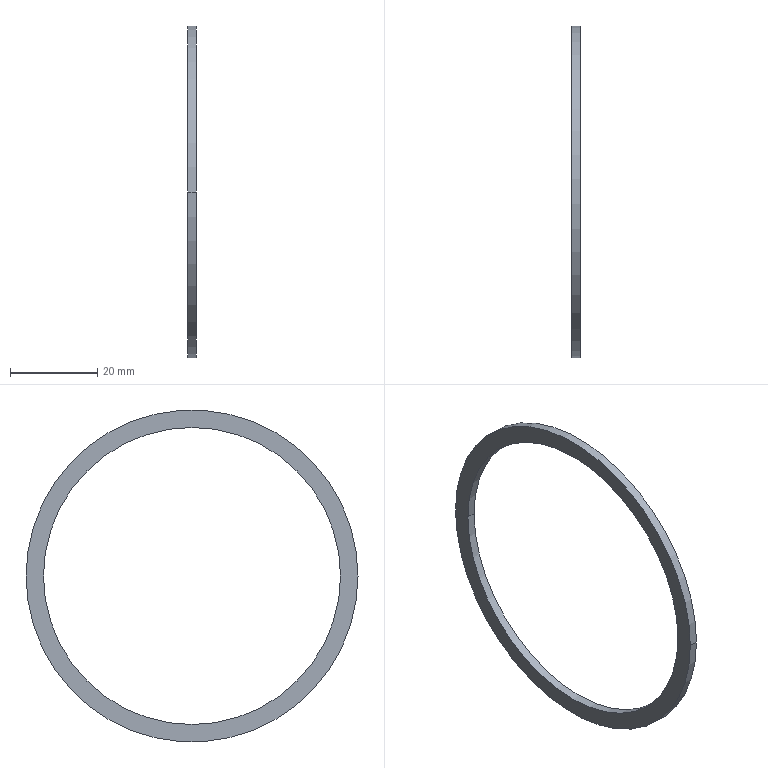Part | NX | features BREP 1 | 1 solid | 6 faces | box 2 x 76 x 76 mm | volume 1810 mm3 | cylinder 4 | plane 2 | commonest cylinder face diameters 68 x2 76 x2
STEP:
#1=CARTESIAN_POINT('',(-550.355,34.,0.));
#2=VERTEX_POINT('',#1);
#3=CARTESIAN_POINT('',(-550.355,-34.,0.));
#4=VERTEX_POINT('',#3);
#5=CARTESIAN_POINT('',(-550.355,0.,0.));
#6=DIRECTION('',(-1.,0.,0.));
#7=DIRECTION('',(0.,-1.,0.));
#8=AXIS2_PLACEMENT_3D('',#5,#6,#7);
#9=CIRCLE('',#8,34.);
#10=EDGE_CURVE('',#2,#4,#9,.T.);
#11=ORIENTED_EDGE('',*,*,#10,.T.);
#12=CARTESIAN_POINT('',(-548.355,-34.,0.));
#13=VERTEX_POINT('',#12);
#14=CARTESIAN_POINT('',(-550.355,-34.,0.));
#15=DIRECTION('',(1.,0.,0.));
#16=VECTOR('',#15,1000.);
#17=LINE('',#14,#16);
#18=EDGE_CURVE('',#4,#13,#17,.T.);
#19=ORIENTED_EDGE('',*,*,#18,.T.);
#20=CARTESIAN_POINT('',(-548.355,34.,0.));
#21=VERTEX_POINT('',#20);
#22=CARTESIAN_POINT('',(-548.355,0.,0.));
#23=DIRECTION('',(-1.,0.,0.));
#24=DIRECTION('',(0.,-1.,0.));
#25=AXIS2_PLACEMENT_3D('',#22,#23,#24);
#26=CIRCLE('',#25,34.);
#27=EDGE_CURVE('',#21,#13,#26,.T.);
#28=ORIENTED_EDGE('',*,*,#27,.F.);
#29=CARTESIAN_POINT('',(-550.355,34.,0.));
#30=DIRECTION('',(1.,0.,0.));
#31=VECTOR('',#30,1000.);
#32=LINE('',#29,#31);
#33=EDGE_CURVE('',#2,#21,#32,.T.);
#34=ORIENTED_EDGE('',*,*,#33,.F.);
#35=EDGE_LOOP('',(#11,#19,#28,#34));
#36=FACE_BOUND('',#35,.T.);
#37=CARTESIAN_POINT('',(-550.355,0.,0.));
#38=DIRECTION('',(1.,0.,0.));
#39=DIRECTION('',(0.,1.,0.));
#40=AXIS2_PLACEMENT_3D('',#37,#38,#39);
#41=CYLINDRICAL_SURFACE('',#40,34.);
#42=ADVANCED_FACE('',(#36),#41,.F.);
#43=CARTESIAN_POINT('',(-550.355,-38.,0.));
#44=VERTEX_POINT('',#43);
#45=CARTESIAN_POINT('',(-550.355,38.,0.));
#46=VERTEX_POINT('',#45);
#47=CARTESIAN_POINT('',(-550.355,0.,0.));
#48=DIRECTION('',(-1.,0.,0.));
#49=DIRECTION('',(0.,-1.,0.));
#50=AXIS2_PLACEMENT_3D('',#47,#48,#49);
#51=CIRCLE('',#50,38.);
#52=EDGE_CURVE('',#44,#46,#51,.T.);
#53=ORIENTED_EDGE('',*,*,#52,.F.);
#54=CARTESIAN_POINT('',(-548.355,-38.,0.));
#55=VERTEX_POINT('',#54);
#56=CARTESIAN_POINT('',(-550.355,-38.,0.));
#57=DIRECTION('',(1.,0.,0.));
#58=VECTOR('',#57,1000.);
#59=LINE('',#56,#58);
#60=EDGE_CURVE('',#44,#55,#59,.T.);
#61=ORIENTED_EDGE('',*,*,#60,.T.);
#62=CARTESIAN_POINT('',(-548.355,38.,0.));
#63=VERTEX_POINT('',#62);
#64=CARTESIAN_POINT('',(-548.355,0.,0.));
#65=DIRECTION('',(-1.,0.,0.));
#66=DIRECTION('',(0.,-1.,0.));
#67=AXIS2_PLACEMENT_3D('',#64,#65,#66);
#68=CIRCLE('',#67,38.);
#69=EDGE_CURVE('',#55,#63,#68,.T.);
#70=ORIENTED_EDGE('',*,*,#69,.T.);
#71=CARTESIAN_POINT('',(-550.355,38.,0.));
#72=DIRECTION('',(1.,0.,0.));
#73=VECTOR('',#72,1000.);
#74=LINE('',#71,#73);
#75=EDGE_CURVE('',#46,#63,#74,.T.);
#76=ORIENTED_EDGE('',*,*,#75,.F.);
#77=EDGE_LOOP('',(#53,#61,#70,#76));
#78=FACE_BOUND('',#77,.T.);
#79=CARTESIAN_POINT('',(-550.355,0.,0.));
#80=DIRECTION('',(1.,0.,0.));
#81=DIRECTION('',(0.,1.,0.));
#82=AXIS2_PLACEMENT_3D('',#79,#80,#81);
#83=CYLINDRICAL_SURFACE('',#82,38.);
#84=ADVANCED_FACE('',(#78),#83,.T.);
#85=CARTESIAN_POINT('',(-550.355,0.,0.));
#86=DIRECTION('',(-1.,0.,0.));
#87=DIRECTION('',(0.,-1.,0.));
#88=AXIS2_PLACEMENT_3D('',#85,#86,#87);
#89=CIRCLE('',#88,38.);
#90=EDGE_CURVE('',#46,#44,#89,.T.);
#91=ORIENTED_EDGE('',*,*,#90,.T.);
#92=ORIENTED_EDGE('',*,*,#52,.T.);
#93=EDGE_LOOP('',(#91,#92));
#94=FACE_BOUND('',#93,.T.);
#95=ORIENTED_EDGE('',*,*,#10,.F.);
#96=CARTESIAN_POINT('',(-550.355,0.,0.));
#97=DIRECTION('',(-1.,0.,0.));
#98=DIRECTION('',(0.,-1.,0.));
#99=AXIS2_PLACEMENT_3D('',#96,#97,#98);
#100=CIRCLE('',#99,34.);
#101=EDGE_CURVE('',#4,#2,#100,.T.);
#102=ORIENTED_EDGE('',*,*,#101,.F.);
#103=EDGE_LOOP('',(#95,#102));
#104=FACE_BOUND('',#103,.T.);
#105=CARTESIAN_POINT('',(-550.355,0.,0.));
#106=DIRECTION('',(-1.,0.,0.));
#107=DIRECTION('',(0.,-1.,0.));
#108=AXIS2_PLACEMENT_3D('',#105,#106,#107);
#109=PLANE('',#108);
#110=ADVANCED_FACE('',(#94,#104),#109,.T.);
#111=CARTESIAN_POINT('',(-548.355,0.,0.));
#112=DIRECTION('',(-1.,0.,0.));
#113=DIRECTION('',(0.,-1.,0.));
#114=AXIS2_PLACEMENT_3D('',#111,#112,#113);
#115=CIRCLE('',#114,38.);
#116=EDGE_CURVE('',#63,#55,#115,.T.);
#117=ORIENTED_EDGE('',*,*,#116,.F.);
#118=ORIENTED_EDGE('',*,*,#69,.F.);
#119=EDGE_LOOP('',(#117,#118));
#120=FACE_BOUND('',#119,.T.);
#121=ORIENTED_EDGE('',*,*,#27,.T.);
#122=CARTESIAN_POINT('',(-548.355,0.,0.));
#123=DIRECTION('',(-1.,0.,0.));
#124=DIRECTION('',(0.,-1.,0.));
#125=AXIS2_PLACEMENT_3D('',#122,#123,#124);
#126=CIRCLE('',#125,34.);
#127=EDGE_CURVE('',#13,#21,#126,.T.);
#128=ORIENTED_EDGE('',*,*,#127,.T.);
#129=EDGE_LOOP('',(#121,#128));
#130=FACE_BOUND('',#129,.T.);
#131=CARTESIAN_POINT('',(-548.355,0.,0.));
#132=DIRECTION('',(-1.,0.,0.));
#133=DIRECTION('',(0.,-1.,0.));
#134=AXIS2_PLACEMENT_3D('',#131,#132,#133);
#135=PLANE('',#134);
#136=ADVANCED_FACE('',(#120,#130),#135,.F.);
#137=ORIENTED_EDGE('',*,*,#60,.F.);
#138=ORIENTED_EDGE('',*,*,#90,.F.);
#139=ORIENTED_EDGE('',*,*,#75,.T.);
#140=ORIENTED_EDGE('',*,*,#116,.T.);
#141=EDGE_LOOP('',(#137,#138,#139,#140));
#142=FACE_BOUND('',#141,.T.);
#143=CARTESIAN_POINT('',(-550.355,0.,0.));
#144=DIRECTION('',(1.,0.,0.));
#145=DIRECTION('',(0.,1.,0.));
#146=AXIS2_PLACEMENT_3D('',#143,#144,#145);
#147=CYLINDRICAL_SURFACE('',#146,38.);
#148=ADVANCED_FACE('',(#142),#147,.T.);
#149=ORIENTED_EDGE('',*,*,#18,.F.);
#150=ORIENTED_EDGE('',*,*,#101,.T.);
#151=ORIENTED_EDGE('',*,*,#33,.T.);
#152=ORIENTED_EDGE('',*,*,#127,.F.);
#153=EDGE_LOOP('',(#149,#150,#151,#152));
#154=FACE_BOUND('',#153,.T.);
#155=CARTESIAN_POINT('',(-550.355,0.,0.));
#156=DIRECTION('',(1.,0.,0.));
#157=DIRECTION('',(0.,1.,0.));
#158=AXIS2_PLACEMENT_3D('',#155,#156,#157);
#159=CYLINDRICAL_SURFACE('',#158,34.);
#160=ADVANCED_FACE('',(#154),#159,.F.);
#161=CLOSED_SHELL('',(#42,#84,#110,#136,#148,#160));
#162=MANIFOLD_SOLID_BREP('',#161);
#163=(LENGTH_UNIT()NAMED_UNIT(*)SI_UNIT(.MILLI.,.METRE.));
#164=UNCERTAINTY_MEASURE_WITH_UNIT(LENGTH_MEASURE(0.00001),#163,'','');
#165=(NAMED_UNIT(*)PLANE_ANGLE_UNIT()SI_UNIT($,.RADIAN.));
#166=(NAMED_UNIT(*)SI_UNIT($,.STERADIAN.)SOLID_ANGLE_UNIT());
#167=(GEOMETRIC_REPRESENTATION_CONTEXT(3)GLOBAL_UNCERTAINTY_ASSIGNED_CONTEXT((#164))GLOBAL_UNIT_ASSIGNED_CONTEXT((#163,#165,#166))REPRESENTATION_CONTEXT('',''));
#168=ADVANCED_BREP_SHAPE_REPRESENTATION('',(#162),#167);